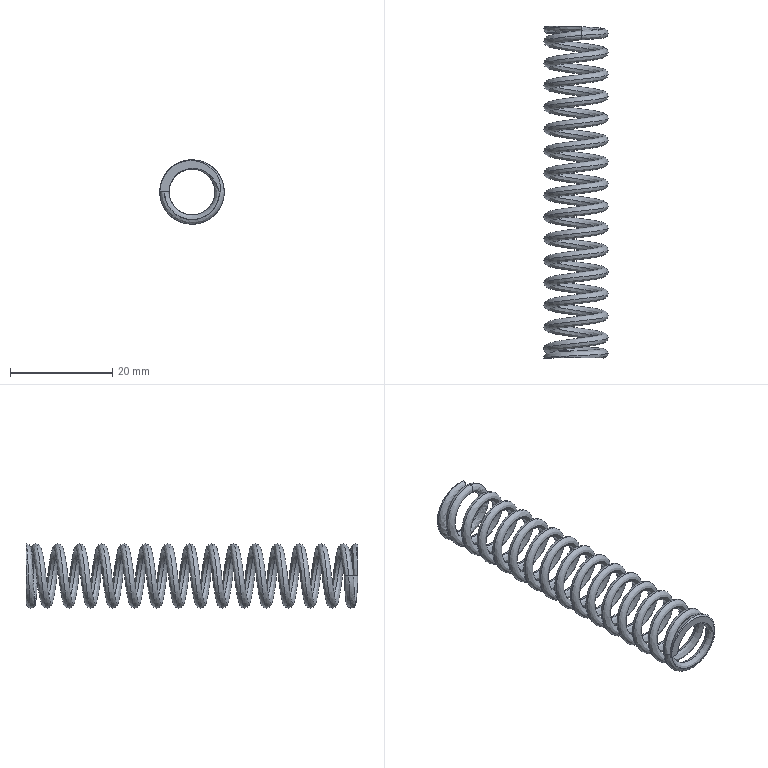Part | SolidWorks | features Sweep 3, ICE 1 | 1 solid | 16 faces | volume 1390 mm3 | spline 12 | plane 4